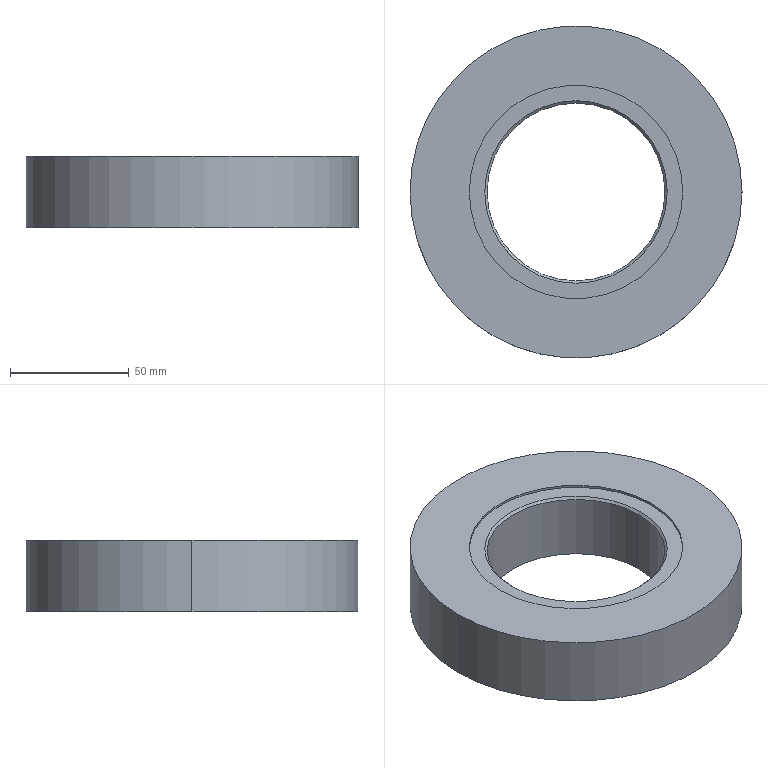Part | SolidWorks | features Chamfer 1, Extrusion 1, ICE 1 | 1 solid | 11 faces | box 140 x 140 x 30 mm | volume 327215 mm3 | cylinder 6 | plane 3 | cone 2 | commonest cylinder face diameters 75 x2 90 x2 140 x2
STEP:
#1=CARTESIAN_POINT('',(-37.5,0.,28.));
#2=VERTEX_POINT('',#1);
#3=CARTESIAN_POINT('',(37.5,0.,28.));
#4=VERTEX_POINT('',#3);
#5=CARTESIAN_POINT('',(0.,0.,28.));
#6=DIRECTION('',(0.,0.,1.));
#7=DIRECTION('',(1.,0.,0.));
#8=AXIS2_PLACEMENT_3D('',#5,#6,#7);
#9=CIRCLE('',#8,37.5);
#10=EDGE_CURVE('',#2,#4,#9,.T.);
#11=ORIENTED_EDGE('',*,*,#10,.F.);
#12=CARTESIAN_POINT('',(-38.5,0.,29.));
#13=VERTEX_POINT('',#12);
#14=CARTESIAN_POINT('',(-37.5,0.,28.));
#15=DIRECTION('',(-0.7071,0.,0.7071));
#16=VECTOR('',#15,1000.);
#17=LINE('',#14,#16);
#18=EDGE_CURVE('',#2,#13,#17,.T.);
#19=ORIENTED_EDGE('',*,*,#18,.T.);
#20=CARTESIAN_POINT('',(38.5,0.,29.));
#21=VERTEX_POINT('',#20);
#22=CARTESIAN_POINT('',(0.,0.,29.));
#23=DIRECTION('',(0.,0.,-1.));
#24=DIRECTION('',(1.,0.,0.));
#25=AXIS2_PLACEMENT_3D('',#22,#23,#24);
#26=CIRCLE('',#25,38.5);
#27=EDGE_CURVE('',#21,#13,#26,.T.);
#28=ORIENTED_EDGE('',*,*,#27,.F.);
#29=CARTESIAN_POINT('',(37.5,0.,28.));
#30=DIRECTION('',(0.7071,0.,0.7071));
#31=VECTOR('',#30,1000.);
#32=LINE('',#29,#31);
#33=EDGE_CURVE('',#4,#21,#32,.T.);
#34=ORIENTED_EDGE('',*,*,#33,.F.);
#35=EDGE_LOOP('',(#11,#19,#28,#34));
#36=FACE_OUTER_BOUND('',#35,.T.);
#37=CARTESIAN_POINT('',(0.,0.,28.));
#38=DIRECTION('',(0.,0.,1.));
#39=DIRECTION('',(1.,0.,0.));
#40=AXIS2_PLACEMENT_3D('',#37,#38,#39);
#41=CONICAL_SURFACE('',#40,37.5,0.7854);
#42=ADVANCED_FACE('',(#36),#41,.F.);
#43=CARTESIAN_POINT('',(-45.,0.,29.));
#44=VERTEX_POINT('',#43);
#45=CARTESIAN_POINT('',(45.,0.,29.));
#46=VERTEX_POINT('',#45);
#47=CARTESIAN_POINT('',(0.,0.,29.));
#48=DIRECTION('',(0.,0.,1.));
#49=DIRECTION('',(1.,0.,0.));
#50=AXIS2_PLACEMENT_3D('',#47,#48,#49);
#51=CIRCLE('',#50,45.);
#52=EDGE_CURVE('',#44,#46,#51,.T.);
#53=ORIENTED_EDGE('',*,*,#52,.F.);
#54=CARTESIAN_POINT('',(-45.,0.,30.));
#55=VERTEX_POINT('',#54);
#56=CARTESIAN_POINT('',(-45.,0.,29.));
#57=DIRECTION('',(0.,0.,1.));
#58=VECTOR('',#57,1000.);
#59=LINE('',#56,#58);
#60=EDGE_CURVE('',#44,#55,#59,.T.);
#61=ORIENTED_EDGE('',*,*,#60,.T.);
#62=CARTESIAN_POINT('',(45.,0.,30.));
#63=VERTEX_POINT('',#62);
#64=CARTESIAN_POINT('',(0.,0.,30.));
#65=DIRECTION('',(0.,0.,1.));
#66=DIRECTION('',(1.,0.,0.));
#67=AXIS2_PLACEMENT_3D('',#64,#65,#66);
#68=CIRCLE('',#67,45.);
#69=EDGE_CURVE('',#55,#63,#68,.T.);
#70=ORIENTED_EDGE('',*,*,#69,.T.);
#71=CARTESIAN_POINT('',(45.,0.,29.));
#72=DIRECTION('',(0.,0.,1.));
#73=VECTOR('',#72,1000.);
#74=LINE('',#71,#73);
#75=EDGE_CURVE('',#46,#63,#74,.T.);
#76=ORIENTED_EDGE('',*,*,#75,.F.);
#77=EDGE_LOOP('',(#53,#61,#70,#76));
#78=FACE_OUTER_BOUND('',#77,.T.);
#79=CARTESIAN_POINT('',(0.,0.,29.));
#80=DIRECTION('',(0.,0.,1.));
#81=DIRECTION('',(1.,0.,0.));
#82=AXIS2_PLACEMENT_3D('',#79,#80,#81);
#83=CYLINDRICAL_SURFACE('',#82,45.);
#84=ADVANCED_FACE('',(#78),#83,.F.);
#85=CARTESIAN_POINT('',(70.,0.,30.));
#86=VERTEX_POINT('',#85);
#87=CARTESIAN_POINT('',(-70.,0.,30.));
#88=VERTEX_POINT('',#87);
#89=CARTESIAN_POINT('',(0.,0.,30.));
#90=DIRECTION('',(0.,0.,1.));
#91=DIRECTION('',(1.,0.,0.));
#92=AXIS2_PLACEMENT_3D('',#89,#90,#91);
#93=CIRCLE('',#92,70.);
#94=EDGE_CURVE('',#86,#88,#93,.T.);
#95=ORIENTED_EDGE('',*,*,#94,.F.);
#96=CARTESIAN_POINT('',(70.,0.,0.));
#97=VERTEX_POINT('',#96);
#98=CARTESIAN_POINT('',(70.,0.,30.));
#99=DIRECTION('',(0.,0.,-1.));
#100=VECTOR('',#99,1000.);
#101=LINE('',#98,#100);
#102=EDGE_CURVE('',#86,#97,#101,.T.);
#103=ORIENTED_EDGE('',*,*,#102,.T.);
#104=CARTESIAN_POINT('',(-70.,0.,0.));
#105=VERTEX_POINT('',#104);
#106=CARTESIAN_POINT('',(0.,0.,0.));
#107=DIRECTION('',(0.,0.,1.));
#108=DIRECTION('',(1.,0.,0.));
#109=AXIS2_PLACEMENT_3D('',#106,#107,#108);
#110=CIRCLE('',#109,70.);
#111=EDGE_CURVE('',#97,#105,#110,.T.);
#112=ORIENTED_EDGE('',*,*,#111,.T.);
#113=CARTESIAN_POINT('',(-70.,0.,30.));
#114=DIRECTION('',(0.,0.,-1.));
#115=VECTOR('',#114,1000.);
#116=LINE('',#113,#115);
#117=EDGE_CURVE('',#88,#105,#116,.T.);
#118=ORIENTED_EDGE('',*,*,#117,.F.);
#119=EDGE_LOOP('',(#95,#103,#112,#118));
#120=FACE_OUTER_BOUND('',#119,.T.);
#121=CARTESIAN_POINT('',(0.,0.,30.));
#122=DIRECTION('',(0.,0.,-1.));
#123=DIRECTION('',(-1.,0.,0.));
#124=AXIS2_PLACEMENT_3D('',#121,#122,#123);
#125=CYLINDRICAL_SURFACE('',#124,70.);
#126=ADVANCED_FACE('',(#120),#125,.T.);
#127=ORIENTED_EDGE('',*,*,#10,.T.);
#128=CARTESIAN_POINT('',(37.5,0.,0.));
#129=VERTEX_POINT('',#128);
#130=CARTESIAN_POINT('',(37.5,0.,30.));
#131=DIRECTION('',(0.,0.,-1.));
#132=VECTOR('',#131,1000.);
#133=LINE('',#130,#132);
#134=EDGE_CURVE('',#4,#129,#133,.T.);
#135=ORIENTED_EDGE('',*,*,#134,.T.);
#136=CARTESIAN_POINT('',(-37.5,0.,0.));
#137=VERTEX_POINT('',#136);
#138=CARTESIAN_POINT('',(0.,0.,0.));
#139=DIRECTION('',(0.,0.,1.));
#140=DIRECTION('',(1.,0.,0.));
#141=AXIS2_PLACEMENT_3D('',#138,#139,#140);
#142=CIRCLE('',#141,37.5);
#143=EDGE_CURVE('',#137,#129,#142,.T.);
#144=ORIENTED_EDGE('',*,*,#143,.F.);
#145=CARTESIAN_POINT('',(-37.5,0.,30.));
#146=DIRECTION('',(0.,0.,-1.));
#147=VECTOR('',#146,1000.);
#148=LINE('',#145,#147);
#149=EDGE_CURVE('',#2,#137,#148,.T.);
#150=ORIENTED_EDGE('',*,*,#149,.F.);
#151=EDGE_LOOP('',(#127,#135,#144,#150));
#152=FACE_OUTER_BOUND('',#151,.T.);
#153=CARTESIAN_POINT('',(0.,0.,30.));
#154=DIRECTION('',(0.,0.,-1.));
#155=DIRECTION('',(-1.,0.,0.));
#156=AXIS2_PLACEMENT_3D('',#153,#154,#155);
#157=CYLINDRICAL_SURFACE('',#156,37.5);
#158=ADVANCED_FACE('',(#152),#157,.F.);
#159=ORIENTED_EDGE('',*,*,#134,.F.);
#160=CARTESIAN_POINT('',(0.,0.,28.));
#161=DIRECTION('',(0.,0.,1.));
#162=DIRECTION('',(1.,0.,0.));
#163=AXIS2_PLACEMENT_3D('',#160,#161,#162);
#164=CIRCLE('',#163,37.5);
#165=EDGE_CURVE('',#4,#2,#164,.T.);
#166=ORIENTED_EDGE('',*,*,#165,.T.);
#167=ORIENTED_EDGE('',*,*,#149,.T.);
#168=CARTESIAN_POINT('',(0.,0.,0.));
#169=DIRECTION('',(0.,0.,1.));
#170=DIRECTION('',(1.,0.,0.));
#171=AXIS2_PLACEMENT_3D('',#168,#169,#170);
#172=CIRCLE('',#171,37.5);
#173=EDGE_CURVE('',#129,#137,#172,.T.);
#174=ORIENTED_EDGE('',*,*,#173,.F.);
#175=EDGE_LOOP('',(#159,#166,#167,#174));
#176=FACE_OUTER_BOUND('',#175,.T.);
#177=CARTESIAN_POINT('',(0.,0.,30.));
#178=DIRECTION('',(0.,0.,-1.));
#179=DIRECTION('',(-1.,0.,0.));
#180=AXIS2_PLACEMENT_3D('',#177,#178,#179);
#181=CYLINDRICAL_SURFACE('',#180,37.5);
#182=ADVANCED_FACE('',(#176),#181,.F.);
#183=CARTESIAN_POINT('',(0.,0.,30.));
#184=DIRECTION('',(0.,0.,1.));
#185=DIRECTION('',(1.,0.,0.));
#186=AXIS2_PLACEMENT_3D('',#183,#184,#185);
#187=CIRCLE('',#186,45.);
#188=EDGE_CURVE('',#63,#55,#187,.T.);
#189=ORIENTED_EDGE('',*,*,#188,.F.);
#190=ORIENTED_EDGE('',*,*,#69,.F.);
#191=EDGE_LOOP('',(#189,#190));
#192=FACE_BOUND('',#191,.T.);
#193=CARTESIAN_POINT('',(0.,0.,30.));
#194=DIRECTION('',(0.,0.,1.));
#195=DIRECTION('',(1.,0.,0.));
#196=AXIS2_PLACEMENT_3D('',#193,#194,#195);
#197=CIRCLE('',#196,70.);
#198=EDGE_CURVE('',#88,#86,#197,.T.);
#199=ORIENTED_EDGE('',*,*,#198,.T.);
#200=ORIENTED_EDGE('',*,*,#94,.T.);
#201=EDGE_LOOP('',(#199,#200));
#202=FACE_OUTER_BOUND('',#201,.T.);
#203=CARTESIAN_POINT('',(0.,0.,30.));
#204=DIRECTION('',(0.,0.,1.));
#205=DIRECTION('',(1.,0.,0.));
#206=AXIS2_PLACEMENT_3D('',#203,#204,#205);
#207=PLANE('',#206);
#208=ADVANCED_FACE('',(#192,#202),#207,.T.);
#209=CARTESIAN_POINT('',(0.,0.,0.));
#210=DIRECTION('',(0.,0.,1.));
#211=DIRECTION('',(1.,0.,0.));
#212=AXIS2_PLACEMENT_3D('',#209,#210,#211);
#213=CIRCLE('',#212,70.);
#214=EDGE_CURVE('',#105,#97,#213,.T.);
#215=ORIENTED_EDGE('',*,*,#214,.F.);
#216=ORIENTED_EDGE('',*,*,#111,.F.);
#217=EDGE_LOOP('',(#215,#216));
#218=FACE_OUTER_BOUND('',#217,.T.);
#219=ORIENTED_EDGE('',*,*,#143,.T.);
#220=ORIENTED_EDGE('',*,*,#173,.T.);
#221=EDGE_LOOP('',(#219,#220));
#222=FACE_BOUND('',#221,.T.);
#223=CARTESIAN_POINT('',(0.,0.,0.));
#224=DIRECTION('',(0.,0.,1.));
#225=DIRECTION('',(1.,0.,0.));
#226=AXIS2_PLACEMENT_3D('',#223,#224,#225);
#227=PLANE('',#226);
#228=ADVANCED_FACE('',(#218,#222),#227,.F.);
#229=ORIENTED_EDGE('',*,*,#102,.F.);
#230=ORIENTED_EDGE('',*,*,#198,.F.);
#231=ORIENTED_EDGE('',*,*,#117,.T.);
#232=ORIENTED_EDGE('',*,*,#214,.T.);
#233=EDGE_LOOP('',(#229,#230,#231,#232));
#234=FACE_OUTER_BOUND('',#233,.T.);
#235=CARTESIAN_POINT('',(0.,0.,30.));
#236=DIRECTION('',(0.,0.,-1.));
#237=DIRECTION('',(-1.,0.,0.));
#238=AXIS2_PLACEMENT_3D('',#235,#236,#237);
#239=CYLINDRICAL_SURFACE('',#238,70.);
#240=ADVANCED_FACE('',(#234),#239,.T.);
#241=ORIENTED_EDGE('',*,*,#60,.F.);
#242=CARTESIAN_POINT('',(0.,0.,29.));
#243=DIRECTION('',(0.,0.,1.));
#244=DIRECTION('',(1.,0.,0.));
#245=AXIS2_PLACEMENT_3D('',#242,#243,#244);
#246=CIRCLE('',#245,45.);
#247=EDGE_CURVE('',#46,#44,#246,.T.);
#248=ORIENTED_EDGE('',*,*,#247,.F.);
#249=ORIENTED_EDGE('',*,*,#75,.T.);
#250=ORIENTED_EDGE('',*,*,#188,.T.);
#251=EDGE_LOOP('',(#241,#248,#249,#250));
#252=FACE_OUTER_BOUND('',#251,.T.);
#253=CARTESIAN_POINT('',(0.,0.,29.));
#254=DIRECTION('',(0.,0.,1.));
#255=DIRECTION('',(1.,0.,0.));
#256=AXIS2_PLACEMENT_3D('',#253,#254,#255);
#257=CYLINDRICAL_SURFACE('',#256,45.);
#258=ADVANCED_FACE('',(#252),#257,.F.);
#259=ORIENTED_EDGE('',*,*,#27,.T.);
#260=CARTESIAN_POINT('',(0.,0.,29.));
#261=DIRECTION('',(0.,0.,-1.));
#262=DIRECTION('',(1.,0.,0.));
#263=AXIS2_PLACEMENT_3D('',#260,#261,#262);
#264=CIRCLE('',#263,38.5);
#265=EDGE_CURVE('',#13,#21,#264,.T.);
#266=ORIENTED_EDGE('',*,*,#265,.T.);
#267=EDGE_LOOP('',(#259,#266));
#268=FACE_BOUND('',#267,.T.);
#269=ORIENTED_EDGE('',*,*,#247,.T.);
#270=ORIENTED_EDGE('',*,*,#52,.T.);
#271=EDGE_LOOP('',(#269,#270));
#272=FACE_OUTER_BOUND('',#271,.T.);
#273=CARTESIAN_POINT('',(0.,0.,29.));
#274=DIRECTION('',(0.,0.,1.));
#275=DIRECTION('',(1.,0.,0.));
#276=AXIS2_PLACEMENT_3D('',#273,#274,#275);
#277=PLANE('',#276);
#278=ADVANCED_FACE('',(#268,#272),#277,.T.);
#279=ORIENTED_EDGE('',*,*,#18,.F.);
#280=ORIENTED_EDGE('',*,*,#165,.F.);
#281=ORIENTED_EDGE('',*,*,#33,.T.);
#282=ORIENTED_EDGE('',*,*,#265,.F.);
#283=EDGE_LOOP('',(#279,#280,#281,#282));
#284=FACE_OUTER_BOUND('',#283,.T.);
#285=CARTESIAN_POINT('',(0.,0.,28.));
#286=DIRECTION('',(0.,0.,1.));
#287=DIRECTION('',(1.,0.,0.));
#288=AXIS2_PLACEMENT_3D('',#285,#286,#287);
#289=CONICAL_SURFACE('',#288,37.5,0.7854);
#290=ADVANCED_FACE('',(#284),#289,.F.);
#291=CLOSED_SHELL('',(#42,#84,#126,#158,#182,#208,#228,#240,#258,#278,#290));
#292=MANIFOLD_SOLID_BREP('',#291);
#293=CARTESIAN_POINT('',(0.,0.,0.));
#294=DIRECTION('',(0.,0.,1.));
#295=DIRECTION('',(1.,0.,0.));
#296=AXIS2_PLACEMENT_3D('',#293,#294,#295);
#297=(LENGTH_UNIT()NAMED_UNIT(*)SI_UNIT(.MILLI.,.METRE.));
#298=UNCERTAINTY_MEASURE_WITH_UNIT(LENGTH_MEASURE(0.00001),#297,'','');
#299=(NAMED_UNIT(*)PLANE_ANGLE_UNIT()SI_UNIT($,.RADIAN.));
#300=(NAMED_UNIT(*)SI_UNIT($,.STERADIAN.)SOLID_ANGLE_UNIT());
#301=(GEOMETRIC_REPRESENTATION_CONTEXT(3)GLOBAL_UNCERTAINTY_ASSIGNED_CONTEXT((#298))GLOBAL_UNIT_ASSIGNED_CONTEXT((#297,#299,#300))REPRESENTATION_CONTEXT('',''));
#302=ADVANCED_BREP_SHAPE_REPRESENTATION('',(#292,#296),#301);